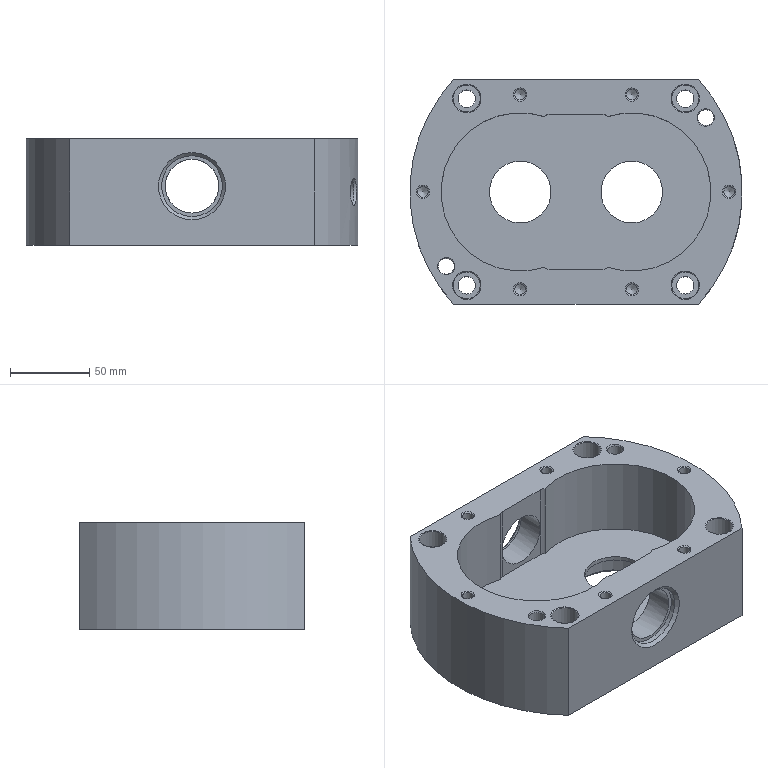NC program | NX | posted with a generic post | part box 210 x 142 x 67.4 mm
Lines 526 to 1432 of 22889:
(FLOOR_WALL_1_1 , TOOL : D25R0.5)
N1032 T05 M6
N1034 G54
N1036 G17 G0 G90 X-2.853 Y1.35 B0. C0. S2000 M3
N1038 G43 Z30. H5
N1040 Z1.5
N1042 G94 G1 X-8.606 Z1.349 F1000.
N1044 X-9.554 Y1.117 Z1.324
N1046 X-12.104 Y0.616 Z1.256
N1048 X-14.678 Y0.256 Z1.188
N1050 X-17.268 Y0.036 Z1.12
N1052 X-18.244 Y0. Z1.094
N1054 X-17.268 Y-0.036 Z1.068
N1056 X-14.678 Y-0.256 Z1.
N1058 X-12.104 Y-0.616 Z0.932
N1060 X-9.554 Y-1.117 Z0.864
N1062 X-8.606 Y-1.35 Z0.839
N1064 X8.606 Z0.388
N1066 X9.554 Y-1.117 Z0.362
N1068 X12.104 Y-0.616 Z0.294
N1070 X14.678 Y-0.256 Z0.226
N1072 X17.268 Y-0.036 Z0.158
N1074 X18.244 Y0. Z0.133
N1076 X17.268 Y0.036 Z0.107
N1078 X14.678 Y0.256 Z0.039
N1080 X12.104 Y0.616 Z-0.029
N1082 X9.554 Y1.117 Z-0.097
N1084 X8.606 Y1.35 Z-0.123
N1086 X0. Z-0.348
N1088 X-8.606 F2200.
N1090 G2 X-18.244 Y0. R47.65
N1092 X-8.606 Y-1.35 R47.65
N1094 G1 X8.606
N1096 G2 X18.244 Y0. R47.65
N1098 X8.606 Y1.35 R47.65
N1100 G1 X0.
N1102 Y18.85
N1104 X-10.975
N1106 G2 X-21.111 Y17.488 R30.15
N1108 G1 X-21.756 Y0.
N1110 G2 X-34.533 Y2.238 R47.65
N1112 G3 X-34.533 Y-2.238 R-2.35
N1114 G2 X-21.756 Y0. R47.65
N1116 G1 X-21.111 Y17.488
N1118 G2 X-29.196 Y18.904 R30.15
N1120 G3 X-29.196 Y-18.904 R-19.85
N1122 G2 X-10.975 Y-18.85 R30.15
N1124 G1 X10.975
N1126 G2 X21.111 Y-17.488 R30.15
N1128 G1 X21.756 Y0.
N1130 G2 X34.533 Y-2.238 R47.65
N1132 G3 X34.533 Y2.238 R-2.35
N1134 G2 X21.756 Y0. R47.65
N1136 G1 X21.111 Y-17.488
N1138 G2 X29.196 Y-18.904 R30.15
N1140 G3 X29.196 Y18.904 R-19.85
N1142 G2 X10.975 Y18.85 R30.15
N1144 G1 X0.
N1146 Y36.35
N1148 X-14.25
N1150 G2 X-23.858 Y35.57 R12.65
N1152 G3 X-23.858 Y-35.57 R-37.35
N1154 G2 X-14.25 Y-36.35 R12.65
N1156 G1 X14.25
N1158 G2 X23.858 Y-35.57 R12.65
N1160 G3 X23.858 Y35.57 R-37.35
N1162 G2 X14.25 Y36.35 R12.65
N1164 G1 X0.
N1166 Z1.152
N1168 G0 X-2.853 Y1.35
N1170 G1 X-8.606 Z1.001 F1000.
N1172 X-9.554 Y1.117 Z0.976
N1174 X-12.104 Y0.616 Z0.908
N1176 X-14.678 Y0.256 Z0.84
N1178 X-17.268 Y0.036 Z0.772
N1180 X-18.244 Y0. Z0.746
N1182 X-17.268 Y-0.036 Z0.721
N1184 X-14.678 Y-0.256 Z0.653
N1186 X-12.104 Y-0.616 Z0.584
N1188 X-9.554 Y-1.117 Z0.516
N1190 X-8.606 Y-1.35 Z0.491
N1192 X8.606 Z0.04
N1194 X9.554 Y-1.117 Z0.015
N1196 X12.104 Y-0.616 Z-0.053
N1198 X14.678 Y-0.256 Z-0.122
N1200 X17.268 Y-0.036 Z-0.19
N1202 X18.244 Y0. Z-0.215
N1204 X17.268 Y0.036 Z-0.241
N1206 X14.678 Y0.256 Z-0.309
N1208 X12.104 Y0.616 Z-0.377
N1210 X9.554 Y1.117 Z-0.445
N1212 X8.606 Y1.35 Z-0.47
N1214 X0. Z-0.696
N1216 X-8.606 F2200.
N1218 G2 X-18.244 Y0. R47.65
N1220 X-8.606 Y-1.35 R47.65
N1222 G1 X8.606
N1224 G2 X18.244 Y0. R47.65
N1226 X8.606 Y1.35 R47.65
N1228 G1 X0.
N1230 Y18.85
N1232 X-10.975
N1234 G2 X-21.111 Y17.488 R30.15
N1236 G1 X-21.756 Y0.
N1238 G2 X-34.533 Y2.238 R47.65
N1240 G3 X-34.533 Y-2.238 R-2.35
N1242 G2 X-21.756 Y0. R47.65
N1244 G1 X-21.111 Y17.488
N1246 G2 X-29.196 Y18.904 R30.15
N1248 G3 X-29.196 Y-18.904 R-19.85
N1250 G2 X-10.975 Y-18.85 R30.15
N1252 G1 X10.975
N1254 G2 X21.111 Y-17.488 R30.15
N1256 G1 X21.756 Y0.
N1258 G2 X34.533 Y-2.238 R47.65
N1260 G3 X34.533 Y2.238 R-2.35
N1262 G2 X21.756 Y0. R47.65
N1264 G1 X21.111 Y-17.488
N1266 G2 X29.196 Y-18.904 R30.15
N1268 G3 X29.196 Y18.904 R-19.85
N1270 G2 X10.975 Y18.85 R30.15
N1272 G1 X0.
N1274 Y36.35
N1276 X-14.25
N1278 G2 X-23.858 Y35.57 R12.65
N1280 G3 X-23.858 Y-35.57 R-37.35
N1282 G2 X-14.25 Y-36.35 R12.65
N1284 G1 X14.25
N1286 G2 X23.858 Y-35.57 R12.65
N1288 G3 X23.858 Y35.57 R-37.35
N1290 G2 X14.25 Y36.35 R12.65
N1292 G1 X0.
N1294 Z0.804
N1296 G0 X-2.853 Y1.35
N1298 G1 X-8.606 Z0.654 F1000.
N1300 X-9.554 Y1.117 Z0.628
N1302 X-12.104 Y0.616 Z0.56
N1304 X-14.678 Y0.256 Z0.492
N1306 X-17.268 Y0.036 Z0.424
N1308 X-18.244 Y0. Z0.398
N1310 X-17.268 Y-0.036 Z0.373
N1312 X-14.678 Y-0.256 Z0.305
N1314 X-12.104 Y-0.616 Z0.237
N1316 X-9.554 Y-1.117 Z0.168
N1318 X-8.606 Y-1.35 Z0.143
N1320 X8.606 Z-0.308
N1322 X9.554 Y-1.117 Z-0.333
N1324 X12.104 Y-0.616 Z-0.401
N1326 X14.678 Y-0.256 Z-0.469
N1328 X17.268 Y-0.036 Z-0.538
N1330 X18.244 Y0. Z-0.563
N1332 X17.268 Y0.036 Z-0.589
N1334 X14.678 Y0.256 Z-0.657
N1336 X12.104 Y0.616 Z-0.725
N1338 X9.554 Y1.117 Z-0.793
N1340 X8.606 Y1.35 Z-0.818
N1342 X0. Z-1.044
N1344 X-8.606 F2200.
N1346 G2 X-18.244 Y0. R47.65
N1348 X-8.606 Y-1.35 R47.65
N1350 G1 X8.606
N1352 G2 X18.244 Y0. R47.65
N1354 X8.606 Y1.35 R47.65
N1356 G1 X0.
N1358 Y18.85
N1360 X-10.975
N1362 G2 X-21.111 Y17.488 R30.15
N1364 G1 X-21.756 Y0.
N1366 G2 X-34.533 Y2.238 R47.65
N1368 G3 X-34.533 Y-2.238 R-2.35
N1370 G2 X-21.756 Y0. R47.65
N1372 G1 X-21.111 Y17.488
N1374 G2 X-29.196 Y18.904 R30.15
N1376 G3 X-29.196 Y-18.904 R-19.85
N1378 G2 X-10.975 Y-18.85 R30.15
N1380 G1 X10.975
N1382 G2 X21.111 Y-17.488 R30.15
N1384 G1 X21.756 Y0.
N1386 G2 X34.533 Y-2.238 R47.65
N1388 G3 X34.533 Y2.238 R-2.35
N1390 G2 X21.756 Y0. R47.65
N1392 G1 X21.111 Y-17.488
N1394 G2 X29.196 Y-18.904 R30.15
N1396 G3 X29.196 Y18.904 R-19.85
N1398 G2 X10.975 Y18.85 R30.15
N1400 G1 X0.
N1402 Y36.35
N1404 X-14.25
N1406 G2 X-23.858 Y35.57 R12.65
N1408 G3 X-23.858 Y-35.57 R-37.35
N1410 G2 X-14.25 Y-36.35 R12.65
N1412 G1 X14.25
N1414 G2 X23.858 Y-35.57 R12.65
N1416 G3 X23.858 Y35.57 R-37.35
N1418 G2 X14.25 Y36.35 R12.65
N1420 G1 X0.
N1422 Z0.456
N1424 G0 X-2.853 Y1.35
N1426 G1 X-8.606 Z0.306 F1000.
N1428 X-9.554 Y1.117 Z0.28
N1430 X-12.104 Y0.616 Z0.212
N1432 X-14.678 Y0.256 Z0.144
N1434 X-17.268 Y0.036 Z0.076
N1436 X-18.244 Y0. Z0.05
N1438 X-17.268 Y-0.036 Z0.025
N1440 X-14.678 Y-0.256 Z-0.043
N1442 X-12.104 Y-0.616 Z-0.111
N1444 X-9.554 Y-1.117 Z-0.179
N1446 X-8.606 Y-1.35 Z-0.205
N1448 X8.606 Z-0.656
N1450 X9.554 Y-1.117 Z-0.681
N1452 X12.104 Y-0.616 Z-0.749
N1454 X14.678 Y-0.256 Z-0.817
N1456 X17.268 Y-0.036 Z-0.885
N1458 X18.244 Y0. Z-0.911
N1460 X17.268 Y0.036 Z-0.937
N1462 X14.678 Y0.256 Z-1.005
N1464 X12.104 Y0.616 Z-1.073
N1466 X9.554 Y1.117 Z-1.141
N1468 X8.606 Y1.35 Z-1.166
N1470 X0. Z-1.392
N1472 X-8.606 F2200.
N1474 G2 X-18.244 Y0. R47.65
N1476 X-8.606 Y-1.35 R47.65
N1478 G1 X8.606
N1480 G2 X18.244 Y0. R47.65
N1482 X8.606 Y1.35 R47.65
N1484 G1 X0.
N1486 Y18.85
N1488 X-10.975
N1490 G2 X-21.111 Y17.488 R30.15
N1492 G1 X-21.756 Y0.
N1494 G2 X-34.533 Y2.238 R47.65
N1496 G3 X-34.533 Y-2.238 R-2.35
N1498 G2 X-21.756 Y0. R47.65
N1500 G1 X-21.111 Y17.488
N1502 G2 X-29.196 Y18.904 R30.15
N1504 G3 X-29.196 Y-18.904 R-19.85
N1506 G2 X-10.975 Y-18.85 R30.15
N1508 G1 X10.975
N1510 G2 X21.111 Y-17.488 R30.15
N1512 G1 X21.756 Y0.
N1514 G2 X34.533 Y-2.238 R47.65
N1516 G3 X34.533 Y2.238 R-2.35
N1518 G2 X21.756 Y0. R47.65
N1520 G1 X21.111 Y-17.488
N1522 G2 X29.196 Y-18.904 R30.15
N1524 G3 X29.196 Y18.904 R-19.85
N1526 G2 X10.975 Y18.85 R30.15
N1528 G1 X0.
N1530 Y36.35
N1532 X-14.25
N1534 G2 X-23.858 Y35.57 R12.65
N1536 G3 X-23.858 Y-35.57 R-37.35
N1538 G2 X-14.25 Y-36.35 R12.65
N1540 G1 X14.25
N1542 G2 X23.858 Y-35.57 R12.65
N1544 G3 X23.858 Y35.57 R-37.35
N1546 G2 X14.25 Y36.35 R12.65
N1548 G1 X0.
N1550 Z0.108
N1552 G0 X-2.853 Y1.35
N1554 G1 X-8.606 Z-0.042 F1000.
N1556 X-9.554 Y1.117 Z-0.068
N1558 X-12.104 Y0.616 Z-0.136
N1560 X-14.678 Y0.256 Z-0.204
N1562 X-17.268 Y0.036 Z-0.272
N1564 X-18.244 Y0. Z-0.298
N1566 X-17.268 Y-0.036 Z-0.323
N1568 X-14.678 Y-0.256 Z-0.391
N1570 X-12.104 Y-0.616 Z-0.459
N1572 X-9.554 Y-1.117 Z-0.527
N1574 X-8.606 Y-1.35 Z-0.553
N1576 X8.606 Z-1.004
N1578 X9.554 Y-1.117 Z-1.029
N1580 X12.104 Y-0.616 Z-1.097
N1582 X14.678 Y-0.256 Z-1.165
N1584 X17.268 Y-0.036 Z-1.233
N1586 X18.244 Y0. Z-1.259
N1588 X17.268 Y0.036 Z-1.284
N1590 X14.678 Y0.256 Z-1.353
N1592 X12.104 Y0.616 Z-1.421
N1594 X9.554 Y1.117 Z-1.489
N1596 X8.606 Y1.35 Z-1.514
N1598 X0. Z-1.74
N1600 X-8.606 F2200.
N1602 G2 X-18.244 Y0. R47.65
N1604 X-8.606 Y-1.35 R47.65
N1606 G1 X8.606
N1608 G2 X18.244 Y0. R47.65
N1610 X8.606 Y1.35 R47.65
N1612 G1 X0.
N1614 Y18.85
N1616 X-10.975
N1618 G2 X-21.111 Y17.488 R30.15
N1620 G1 X-21.756 Y0.
N1622 G2 X-34.533 Y2.238 R47.65
N1624 G3 X-34.533 Y-2.238 R-2.35
N1626 G2 X-21.756 Y0. R47.65
N1628 G1 X-21.111 Y17.488
N1630 G2 X-29.196 Y18.904 R30.15
N1632 G3 X-29.196 Y-18.904 R-19.85
N1634 G2 X-10.975 Y-18.85 R30.15
N1636 G1 X10.975
N1638 G2 X21.111 Y-17.488 R30.15
N1640 G1 X21.756 Y0.
N1642 G2 X34.533 Y-2.238 R47.65
N1644 G3 X34.533 Y2.238 R-2.35
N1646 G2 X21.756 Y0. R47.65
N1648 G1 X21.111 Y-17.488
N1650 G2 X29.196 Y-18.904 R30.15
N1652 G3 X29.196 Y18.904 R-19.85
N1654 G2 X10.975 Y18.85 R30.15
N1656 G1 X0.
N1658 Y36.35
N1660 X-14.25
N1662 G2 X-23.858 Y35.57 R12.65
N1664 G3 X-23.858 Y-35.57 R-37.35
N1666 G2 X-14.25 Y-36.35 R12.65
N1668 G1 X14.25
N1670 G2 X23.858 Y-35.57 R12.65
N1672 G3 X23.858 Y35.57 R-37.35
N1674 G2 X14.25 Y36.35 R12.65
N1676 G1 X0.
N1678 Z-0.24
N1680 G0 X-2.853 Y1.35
N1682 G1 X-8.606 Z-0.39 F1000.
N1684 X-9.554 Y1.117 Z-0.416
N1686 X-12.104 Y0.616 Z-0.484
N1688 X-14.678 Y0.256 Z-0.552
N1690 X-17.268 Y0.036 Z-0.62
N1692 X-18.244 Y0. Z-0.646
N1694 X-17.268 Y-0.036 Z-0.671
N1696 X-14.678 Y-0.256 Z-0.739
N1698 X-12.104 Y-0.616 Z-0.807
N1700 X-9.554 Y-1.117 Z-0.875
N1702 X-8.606 Y-1.35 Z-0.901
N1704 X8.606 Z-1.352
N1706 X9.554 Y-1.117 Z-1.377
N1708 X12.104 Y-0.616 Z-1.445
N1710 X14.678 Y-0.256 Z-1.513
N1712 X17.268 Y-0.036 Z-1.581
N1714 X18.244 Y0. Z-1.607
N1716 X17.268 Y0.036 Z-1.632
N1718 X14.678 Y0.256 Z-1.7
N1720 X12.104 Y0.616 Z-1.769
N1722 X9.554 Y1.117 Z-1.837
N1724 X8.606 Y1.35 Z-1.862
N1726 X0. Z-2.088
N1728 X-8.606 F2200.
N1730 G2 X-18.244 Y0. R47.65
N1732 X-8.606 Y-1.35 R47.65
N1734 G1 X8.606
N1736 G2 X18.244 Y0. R47.65
N1738 X8.606 Y1.35 R47.65
N1740 G1 X0.
N1742 Y18.85
N1744 X-10.975
N1746 G2 X-21.111 Y17.488 R30.15
N1748 G1 X-21.756 Y0.
N1750 G2 X-34.533 Y2.238 R47.65
N1752 G3 X-34.533 Y-2.238 R-2.35
N1754 G2 X-21.756 Y0. R47.65
N1756 G1 X-21.111 Y17.488
N1758 G2 X-29.196 Y18.904 R30.15
N1760 G3 X-29.196 Y-18.904 R-19.85
N1762 G2 X-10.975 Y-18.85 R30.15
N1764 G1 X10.975
N1766 G2 X21.111 Y-17.488 R30.15
N1768 G1 X21.756 Y0.
N1770 G2 X34.533 Y-2.238 R47.65
N1772 G3 X34.533 Y2.238 R-2.35
N1774 G2 X21.756 Y0. R47.65
N1776 G1 X21.111 Y-17.488
N1778 G2 X29.196 Y-18.904 R30.15
N1780 G3 X29.196 Y18.904 R-19.85
N1782 G2 X10.975 Y18.85 R30.15
N1784 G1 X0.
N1786 Y36.35
N1788 X-14.25
N1790 G2 X-23.858 Y35.57 R12.65
N1792 G3 X-23.858 Y-35.57 R-37.35
N1794 G2 X-14.25 Y-36.35 R12.65
N1796 G1 X14.25
N1798 G2 X23.858 Y-35.57 R12.65
N1800 G3 X23.858 Y35.57 R-37.35
N1802 G2 X14.25 Y36.35 R12.65
N1804 G1 X0.
N1806 Z-0.588
N1808 G0 X-2.853 Y1.35
N1810 G1 X-8.606 Z-0.738 F1000.
N1812 X-9.554 Y1.117 Z-0.764
N1814 X-12.104 Y0.616 Z-0.832
N1816 X-14.678 Y0.256 Z-0.9
N1818 X-17.268 Y0.036 Z-0.968
N1820 X-18.244 Y0. Z-0.993
N1822 X-17.268 Y-0.036 Z-1.019
N1824 X-14.678 Y-0.256 Z-1.087
N1826 X-12.104 Y-0.616 Z-1.155
N1828 X-9.554 Y-1.117 Z-1.223
N1830 X-8.606 Y-1.35 Z-1.249
N1832 X8.606 Z-1.699
N1834 X9.554 Y-1.117 Z-1.725
N1836 X12.104 Y-0.616 Z-1.793
N1838 X14.678 Y-0.256 Z-1.861
N1840 X17.268 Y-0.036 Z-1.929
N1842 X18.244 Y0. Z-1.955
N1844 X17.268 Y0.036 Z-1.98
N1846 X14.678 Y0.256 Z-2.048
N1848 X12.104 Y0.616 Z-2.116
N1850 X9.554 Y1.117 Z-2.185
N1852 X8.606 Y1.35 Z-2.21
N1854 X0. Z-2.435
N1856 X-8.606 F2200.
N1858 G2 X-18.244 Y0. R47.65
N1860 X-8.606 Y-1.35 R47.65
N1862 G1 X8.606
N1864 G2 X18.244 Y0. R47.65
N1866 X8.606 Y1.35 R47.65
N1868 G1 X0.
N1870 Y18.85
N1872 X-10.975
N1874 G2 X-21.111 Y17.488 R30.15
N1876 G1 X-21.756 Y0.
N1878 G2 X-34.533 Y2.238 R47.65
N1880 G3 X-34.533 Y-2.238 R-2.35
N1882 G2 X-21.756 Y0. R47.65
N1884 G1 X-21.111 Y17.488
N1886 G2 X-29.196 Y18.904 R30.15
N1888 G3 X-29.196 Y-18.904 R-19.85
N1890 G2 X-10.975 Y-18.85 R30.15
N1892 G1 X10.975
N1894 G2 X21.111 Y-17.488 R30.15
N1896 G1 X21.756 Y0.
N1898 G2 X34.533 Y-2.238 R47.65
N1900 G3 X34.533 Y2.238 R-2.35
N1902 G2 X21.756 Y0. R47.65
N1904 G1 X21.111 Y-17.488
N1906 G2 X29.196 Y-18.904 R30.15
N1908 G3 X29.196 Y18.904 R-19.85
N1910 G2 X10.975 Y18.85 R30.15
N1912 G1 X0.
N1914 Y36.35
N1916 X-14.25
N1918 G2 X-23.858 Y35.57 R12.65
N1920 G3 X-23.858 Y-35.57 R-37.35
N1922 G2 X-14.25 Y-36.35 R12.65
N1924 G1 X14.25
N1926 G2 X23.858 Y-35.57 R12.65
N1928 G3 X23.858 Y35.57 R-37.35
N1930 G2 X14.25 Y36.35 R12.65
N1932 G1 X0.
N1934 Z-0.935
N1936 G0 X-2.853 Y1.35
N1938 G1 X-8.606 Z-1.086 F1000.
N1940 X-9.554 Y1.117 Z-1.112
N1942 X-12.104 Y0.616 Z-1.18
N1944 X-14.678 Y0.256 Z-1.248
N1946 X-17.268 Y0.036 Z-1.316
N1948 X-18.244 Y0. Z-1.341
N1950 X-17.268 Y-0.036 Z-1.367
N1952 X-14.678 Y-0.256 Z-1.435
N1954 X-12.104 Y-0.616 Z-1.503
N1956 X-9.554 Y-1.117 Z-1.571
N1958 X-8.606 Y-1.35 Z-1.597
N1960 X8.606 Z-2.047
N1962 X9.554 Y-1.117 Z-2.073
N1964 X12.104 Y-0.616 Z-2.141
N1966 X14.678 Y-0.256 Z-2.209
N1968 X17.268 Y-0.036 Z-2.277
N1970 X18.244 Y0. Z-2.303
N1972 X17.268 Y0.036 Z-2.328
N1974 X14.678 Y0.256 Z-2.396
N1976 X12.104 Y0.616 Z-2.464
N1978 X9.554 Y1.117 Z-2.532
N1980 X8.606 Y1.35 Z-2.558
N1982 X0. Z-2.783
N1984 X-8.606 F2200.
N1986 G2 X-18.244 Y0. R47.65
N1988 X-8.606 Y-1.35 R47.65
N1990 G1 X8.606
N1992 G2 X18.244 Y0. R47.65
N1994 X8.606 Y1.35 R47.65
N1996 G1 X0.
N1998 Y18.85
N2000 X-10.975
N2002 G2 X-21.111 Y17.488 R30.15
N2004 G1 X-21.756 Y0.
N2006 G2 X-34.533 Y2.238 R47.65
N2008 G3 X-34.533 Y-2.238 R-2.35
N2010 G2 X-21.756 Y0. R47.65
N2012 G1 X-21.111 Y17.488
N2014 G2 X-29.196 Y18.904 R30.15
N2016 G3 X-29.196 Y-18.904 R-19.85
N2018 G2 X-10.975 Y-18.85 R30.15
N2020 G1 X10.975
N2022 G2 X21.111 Y-17.488 R30.15
N2024 G1 X21.756 Y0.
N2026 G2 X34.533 Y-2.238 R47.65
N2028 G3 X34.533 Y2.238 R-2.35
N2030 G2 X21.756 Y0. R47.65
N2032 G1 X21.111 Y-17.488
N2034 G2 X29.196 Y-18.904 R30.15
N2036 G3 X29.196 Y18.904 R-19.85
N2038 G2 X10.975 Y18.85 R30.15
N2040 G1 X0.
N2042 Y36.35
N2044 X-14.25
N2046 G2 X-23.858 Y35.57 R12.65
N2048 G3 X-23.858 Y-35.57 R-37.35
N2050 G2 X-14.25 Y-36.35 R12.65
N2052 G1 X14.25
N2054 G2 X23.858 Y-35.57 R12.65
N2056 G3 X23.858 Y35.57 R-37.35
N2058 G2 X14.25 Y36.35 R12.65
N2060 G1 X0.
N2062 Z-1.283
N2064 G0 X-2.853 Y1.35
N2066 G1 X-8.606 Z-1.434 F1000.
N2068 X-9.554 Y1.117 Z-1.46
N2070 X-12.104 Y0.616 Z-1.528
N2072 X-14.678 Y0.256 Z-1.596
N2074 X-17.268 Y0.036 Z-1.664
N2076 X-18.244 Y0. Z-1.689
N2078 X-17.268 Y-0.036 Z-1.715
N2080 X-14.678 Y-0.256 Z-1.783
N2082 X-12.104 Y-0.616 Z-1.851
N2084 X-9.554 Y-1.117 Z-1.919
N2086 X-8.606 Y-1.35 Z-1.945
N2088 X8.606 Z-2.395
N2090 X9.554 Y-1.117 Z-2.421
N2092 X12.104 Y-0.616 Z-2.489
N2094 X14.678 Y-0.256 Z-2.557
N2096 X17.268 Y-0.036 Z-2.625
N2098 X18.244 Y0. Z-2.651
N2100 X17.268 Y0.036 Z-2.676
N2102 X14.678 Y0.256 Z-2.744
N2104 X12.104 Y0.616 Z-2.812
N2106 X9.554 Y1.117 Z-2.88
N2108 X8.606 Y1.35 Z-2.906
N2110 X0. Z-3.131
N2112 X-8.606 F2200.
N2114 G2 X-18.244 Y0. R47.65
N2116 X-8.606 Y-1.35 R47.65
N2118 G1 X8.606
N2120 G2 X18.244 Y0. R47.65
N2122 X8.606 Y1.35 R47.65
N2124 G1 X0.
N2126 Y18.85
N2128 X-10.975
N2130 G2 X-21.111 Y17.488 R30.15
N2132 G1 X-21.756 Y0.
N2134 G2 X-34.533 Y2.238 R47.65
N2136 G3 X-34.533 Y-2.238 R-2.35
N2138 G2 X-21.756 Y0. R47.65
N2140 G1 X-21.111 Y17.488
N2142 G2 X-29.196 Y18.904 R30.15
N2144 G3 X-29.196 Y-18.904 R-19.85
N2146 G2 X-10.975 Y-18.85 R30.15
N2148 G1 X10.975
N2150 G2 X21.111 Y-17.488 R30.15
N2152 G1 X21.756 Y0.
N2154 G2 X34.533 Y-2.238 R47.65
N2156 G3 X34.533 Y2.238 R-2.35
N2158 G2 X21.756 Y0. R47.65
N2160 G1 X21.111 Y-17.488
N2162 G2 X29.196 Y-18.904 R30.15
N2164 G3 X29.196 Y18.904 R-19.85
N2166 G2 X10.975 Y18.85 R30.15
N2168 G1 X0.
N2170 Y36.35
N2172 X-14.25
N2174 G2 X-23.858 Y35.57 R12.65
N2176 G3 X-23.858 Y-35.57 R-37.35
N2178 G2 X-14.25 Y-36.35 R12.65
N2180 G1 X14.25
N2182 G2 X23.858 Y-35.57 R12.65
N2184 G3 X23.858 Y35.57 R-37.35
N2186 G2 X14.25 Y36.35 R12.65
N2188 G1 X0.
N2190 Z-1.631
N2192 G0 X-2.853 Y1.35
N2194 G1 X-8.606 Z-1.782 F1000.
N2196 X-9.554 Y1.117 Z-1.807
N2198 X-12.104 Y0.616 Z-1.876
N2200 X-14.678 Y0.256 Z-1.944
N2202 X-17.268 Y0.036 Z-2.012
N2204 X-18.244 Y0. Z-2.037
N2206 X-17.268 Y-0.036 Z-2.063
N2208 X-14.678 Y-0.256 Z-2.131
N2210 X-12.104 Y-0.616 Z-2.199
N2212 X-9.554 Y-1.117 Z-2.267
N2214 X-8.606 Y-1.35 Z-2.293
N2216 X8.606 Z-2.743
N2218 X9.554 Y-1.117 Z-2.769
N2220 X12.104 Y-0.616 Z-2.837
N2222 X14.678 Y-0.256 Z-2.905
N2224 X17.268 Y-0.036 Z-2.973
N2226 X18.244 Y0. Z-2.999
N2228 X17.268 Y0.036 Z-3.024
N2230 X14.678 Y0.256 Z-3.092
N2232 X12.104 Y0.616 Z-3.16
N2234 X9.554 Y1.117 Z-3.228
N2236 X8.606 Y1.35 Z-3.254
N2238 X0. Z-3.479
N2240 X-8.606 F2200.
N2242 G2 X-18.244 Y0. R47.65
N2244 X-8.606 Y-1.35 R47.65
N2246 G1 X8.606
N2248 G2 X18.244 Y0. R47.65
N2250 X8.606 Y1.35 R47.65
N2252 G1 X0.
N2254 Y18.85
N2256 X-10.975
N2258 G2 X-21.111 Y17.488 R30.15
N2260 G1 X-21.756 Y0.
N2262 G2 X-34.533 Y2.238 R47.65
N2264 G3 X-34.533 Y-2.238 R-2.35
N2266 G2 X-21.756 Y0. R47.65
N2268 G1 X-21.111 Y17.488
N2270 G2 X-29.196 Y18.904 R30.15
N2272 G3 X-29.196 Y-18.904 R-19.85
N2274 G2 X-10.975 Y-18.85 R30.15
N2276 G1 X10.975
N2278 G2 X21.111 Y-17.488 R30.15
N2280 G1 X21.756 Y0.
N2282 G2 X34.533 Y-2.238 R47.65
N2284 G3 X34.533 Y2.238 R-2.35
N2286 G2 X21.756 Y0. R47.65
N2288 G1 X21.111 Y-17.488
N2290 G2 X29.196 Y-18.904 R30.15
N2292 G3 X29.196 Y18.904 R-19.85
N2294 G2 X10.975 Y18.85 R30.15
N2296 G1 X0.
N2298 Y36.35
N2300 X-14.25
N2302 G2 X-23.858 Y35.57 R12.65
N2304 G3 X-23.858 Y-35.57 R-37.35
N2306 G2 X-14.25 Y-36.35 R12.65
N2308 G1 X14.25
N2310 G2 X23.858 Y-35.57 R12.65
N2312 G3 X23.858 Y35.57 R-37.35
N2314 G2 X14.25 Y36.35 R12.65
N2316 G1 X0.
N2318 Z-1.979
N2320 G0 X-2.853 Y1.35
N2322 G1 X-8.606 Z-2.13 F1000.
N2324 X-9.554 Y1.117 Z-2.155
N2326 X-12.104 Y0.616 Z-2.223
N2328 X-14.678 Y0.256 Z-2.291
N2330 X-17.268 Y0.036 Z-2.36
N2332 X-18.244 Y0. Z-2.385
N2334 X-17.268 Y-0.036 Z-2.411
N2336 X-14.678 Y-0.256 Z-2.479
N2338 X-12.104 Y-0.616 Z-2.547
N2340 X-9.554 Y-1.117 Z-2.615
N2342 X-8.606 Y-1.35 Z-2.64
N2344 X8.606 Z-3.091
N2346 X9.554 Y-1.117 Z-3.117
N2348 X12.104 Y-0.616 Z-3.185
N2350 X14.678 Y-0.256 Z-3.253
N2352 X17.268 Y-0.036 Z-3.321
N2354 X18.244 Y0. Z-3.346
N2356 X17.268 Y0.036 Z-3.372
N2358 X14.678 Y0.256 Z-3.44
N2360 X12.104 Y0.616 Z-3.508
N2362 X9.554 Y1.117 Z-3.576
N2364 X8.606 Y1.35 Z-3.602
N2366 X0. Z-3.827
N2368 X-8.606 F2200.
N2370 G2 X-18.244 Y0. R47.65
N2372 X-8.606 Y-1.35 R47.65
N2374 G1 X8.606
N2376 G2 X18.244 Y0. R47.65
N2378 X8.606 Y1.35 R47.65
N2380 G1 X0.
N2382 Y18.85
N2384 X-10.975
N2386 G2 X-21.111 Y17.488 R30.15
N2388 G1 X-21.756 Y0.
N2390 G2 X-34.533 Y2.238 R47.65
N2392 G3 X-34.533 Y-2.238 R-2.35
N2394 G2 X-21.756 Y0. R47.65
N2396 G1 X-21.111 Y17.488
N2398 G2 X-29.196 Y18.904 R30.15
N2400 G3 X-29.196 Y-18.904 R-19.85
N2402 G2 X-10.975 Y-18.85 R30.15
N2404 G1 X10.975
N2406 G2 X21.111 Y-17.488 R30.15
N2408 G1 X21.756 Y0.
N2410 G2 X34.533 Y-2.238 R47.65
N2412 G3 X34.533 Y2.238 R-2.35
N2414 G2 X21.756 Y0. R47.65
N2416 G1 X21.111 Y-17.488
N2418 G2 X29.196 Y-18.904 R30.15
N2420 G3 X29.196 Y18.904 R-19.85
N2422 G2 X10.975 Y18.85 R30.15
N2424 G1 X0.
N2426 Y36.35
N2428 X-14.25
N2430 G2 X-23.858 Y35.57 R12.65
N2432 G3 X-23.858 Y-35.57 R-37.35
N2434 G2 X-14.25 Y-36.35 R12.65
N2436 G1 X14.25
N2438 G2 X23.858 Y-35.57 R12.65
N2440 G3 X23.858 Y35.57 R-37.35
N2442 G2 X14.25 Y36.35 R12.65
N2444 G1 X0.
N2446 Z-2.327
N2448 G0 X-2.853 Y1.35
N2450 G1 X-8.606 Z-2.478 F1000.
N2452 X-9.554 Y1.117 Z-2.503
N2454 X-12.104 Y0.616 Z-2.571
N2456 X-14.678 Y0.256 Z-2.639
N2458 X-17.268 Y0.036 Z-2.707
N2460 X-18.244 Y0. Z-2.733
N2462 X-17.268 Y-0.036 Z-2.759
N2464 X-14.678 Y-0.256 Z-2.827
N2466 X-12.104 Y-0.616 Z-2.895
N2468 X-9.554 Y-1.117 Z-2.963
N2470 X-8.606 Y-1.35 Z-2.988
N2472 X8.606 Z-3.439
N2474 X9.554 Y-1.117 Z-3.465
N2476 X12.104 Y-0.616 Z-3.533
N2478 X14.678 Y-0.256 Z-3.601
N2480 X17.268 Y-0.036 Z-3.669
N2482 X18.244 Y0. Z-3.694
N2484 X17.268 Y0.036 Z-3.72
N2486 X14.678 Y0.256 Z-3.788
N2488 X12.104 Y0.616 Z-3.856
N2490 X9.554 Y1.117 Z-3.924
N2492 X8.606 Y1.35 Z-3.95
N2494 X0. Z-4.175
N2496 X-8.606 F2200.
N2498 G2 X-18.244 Y0. R47.65
N2500 X-8.606 Y-1.35 R47.65
N2502 G1 X8.606
N2504 G2 X18.244 Y0. R47.65
N2506 X8.606 Y1.35 R47.65
N2508 G1 X0.
N2510 Y18.85
N2512 X-10.975
N2514 G2 X-21.111 Y17.488 R30.15
N2516 G1 X-21.756 Y0.
N2518 G2 X-34.533 Y2.238 R47.65
N2520 G3 X-34.533 Y-2.238 R-2.35
N2522 G2 X-21.756 Y0. R47.65
N2524 G1 X-21.111 Y17.488
N2526 G2 X-29.196 Y18.904 R30.15
N2528 G3 X-29.196 Y-18.904 R-19.85
N2530 G2 X-10.975 Y-18.85 R30.15
N2532 G1 X10.975
N2534 G2 X21.111 Y-17.488 R30.15
N2536 G1 X21.756 Y0.
N2538 G2 X34.533 Y-2.238 R47.65
N2540 G3 X34.533 Y2.238 R-2.35
N2542 G2 X21.756 Y0. R47.65
N2544 G1 X21.111 Y-17.488
N2546 G2 X29.196 Y-18.904 R30.15
N2548 G3 X29.196 Y18.904 R-19.85
N2550 G2 X10.975 Y18.85 R30.15
N2552 G1 X0.
N2554 Y36.35
N2556 X-14.25
N2558 G2 X-23.858 Y35.57 R12.65
N2560 G3 X-23.858 Y-35.57 R-37.35
N2562 G2 X-14.25 Y-36.35 R12.65
N2564 G1 X14.25
N2566 G2 X23.858 Y-35.57 R12.65
N2568 G3 X23.858 Y35.57 R-37.35
N2570 G2 X14.25 Y36.35 R12.65
N2572 G1 X0.
N2574 Z-2.675
N2576 G0 X-2.853 Y1.35
N2578 G1 X-8.606 Z-2.826 F1000.
N2580 X-9.554 Y1.117 Z-2.851
N2582 X-12.104 Y0.616 Z-2.919
N2584 X-14.678 Y0.256 Z-2.987
N2586 X-17.268 Y0.036 Z-3.055
N2588 X-18.244 Y0. Z-3.081
N2590 X-17.268 Y-0.036 Z-3.107
N2592 X-14.678 Y-0.256 Z-3.175
N2594 X-12.104 Y-0.616 Z-3.243
N2596 X-9.554 Y-1.117 Z-3.311
N2598 X-8.606 Y-1.35 Z-3.336
N2600 X8.606 Z-3.787
N2602 X9.554 Y-1.117 Z-3.813
N2604 X12.104 Y-0.616 Z-3.881
N2606 X14.678 Y-0.256 Z-3.949
N2608 X17.268 Y-0.036 Z-4.017
N2610 X18.244 Y0. Z-4.042
N2612 X17.268 Y0.036 Z-4.068
N2614 X14.678 Y0.256 Z-4.136
N2616 X12.104 Y0.616 Z-4.204
N2618 X9.554 Y1.117 Z-4.272
N2620 X8.606 Y1.35 Z-4.298
N2622 X0. Z-4.523
N2624 X-8.606 F2200.
N2626 G2 X-18.244 Y0. R47.65
N2628 X-8.606 Y-1.35 R47.65
N2630 G1 X8.606
N2632 G2 X18.244 Y0. R47.65
N2634 X8.606 Y1.35 R47.65
N2636 G1 X0.
N2638 Y18.85
N2640 X-10.975
N2642 G2 X-21.111 Y17.488 R30.15
N2644 G1 X-21.756 Y0.
N2646 G2 X-34.533 Y2.238 R47.65
N2648 G3 X-34.533 Y-2.238 R-2.35
N2650 G2 X-21.756 Y0. R47.65
N2652 G1 X-21.111 Y17.488
N2654 G2 X-29.196 Y18.904 R30.15
N2656 G3 X-29.196 Y-18.904 R-19.85
N2658 G2 X-10.975 Y-18.85 R30.15
N2660 G1 X10.975
N2662 G2 X21.111 Y-17.488 R30.15
N2664 G1 X21.756 Y0.
N2666 G2 X34.533 Y-2.238 R47.65
N2668 G3 X34.533 Y2.238 R-2.35
N2670 G2 X21.756 Y0. R47.65
N2672 G1 X21.111 Y-17.488
N2674 G2 X29.196 Y-18.904 R30.15
N2676 G3 X29.196 Y18.904 R-19.85
N2678 G2 X10.975 Y18.85 R30.15
N2680 G1 X0.
N2682 Y36.35
N2684 X-14.25
N2686 G2 X-23.858 Y35.57 R12.65
N2688 G3 X-23.858 Y-35.57 R-37.35
N2690 G2 X-14.25 Y-36.35 R12.65
N2692 G1 X14.25
N2694 G2 X23.858 Y-35.57 R12.65
N2696 G3 X23.858 Y35.57 R-37.35
N2698 G2 X14.25 Y36.35 R12.65
N2700 G1 X0.
N2702 Z-3.023
N2704 G0 X-2.853 Y1.35
N2706 G1 X-8.606 Z-3.174 F1000.
N2708 X-9.554 Y1.117 Z-3.199
N2710 X-12.104 Y0.616 Z-3.267
N2712 X-14.678 Y0.256 Z-3.335
N2714 X-17.268 Y0.036 Z-3.403
N2716 X-18.244 Y0. Z-3.429
N2718 X-17.268 Y-0.036 Z-3.454
N2720 X-14.678 Y-0.256 Z-3.522
N2722 X-12.104 Y-0.616 Z-3.591
N2724 X-9.554 Y-1.117 Z-3.659
N2726 X-8.606 Y-1.35 Z-3.684
N2728 X8.606 Z-4.135
N2730 X9.554 Y-1.117 Z-4.16
N2732 X12.104 Y-0.616 Z-4.228
N2734 X14.678 Y-0.256 Z-4.297
N2736 X17.268 Y-0.036 Z-4.365
N2738 X18.244 Y0. Z-4.39
N2740 X17.268 Y0.036 Z-4.416
N2742 X14.678 Y0.256 Z-4.484
N2744 X12.104 Y0.616 Z-4.552
N2746 X9.554 Y1.117 Z-4.62
N2748 X8.606 Y1.35 Z-4.645
N2750 X0. Z-4.871
N2752 X-8.606 F2200.
N2754 G2 X-18.244 Y0. R47.65
N2756 X-8.606 Y-1.35 R47.65
N2758 G1 X8.606
N2760 G2 X18.244 Y0. R47.65
N2762 X8.606 Y1.35 R47.65
N2764 G1 X0.
N2766 Y18.85
N2768 X-10.975
N2770 G2 X-21.111 Y17.488 R30.15
N2772 G1 X-21.756 Y0.
N2774 G2 X-34.533 Y2.238 R47.65
N2776 G3 X-34.533 Y-2.238 R-2.35
N2778 G2 X-21.756 Y0. R47.65
N2780 G1 X-21.111 Y17.488
N2782 G2 X-29.196 Y18.904 R30.15
N2784 G3 X-29.196 Y-18.904 R-19.85
N2786 G2 X-10.975 Y-18.85 R30.15
N2788 G1 X10.975
N2790 G2 X21.111 Y-17.488 R30.15
N2792 G1 X21.756 Y0.
N2794 G2 X34.533 Y-2.238 R47.65
N2796 G3 X34.533 Y2.238 R-2.35
N2798 G2 X21.756 Y0. R47.65
N2800 G1 X21.111 Y-17.488
N2802 G2 X29.196 Y-18.904 R30.15
N2804 G3 X29.196 Y18.904 R-19.85
N2806 G2 X10.975 Y18.85 R30.15
N2808 G1 X0.
N2810 Y36.35
N2812 X-14.25
N2814 G2 X-23.858 Y35.57 R12.65
N2816 G3 X-23.858 Y-35.57 R-37.35
N2818 G2 X-14.25 Y-36.35 R12.65
N2820 G1 X14.25
N2822 G2 X23.858 Y-35.57 R12.65
N2824 G3 X23.858 Y35.57 R-37.35
N2826 G2 X14.25 Y36.35 R12.65
N2828 G1 X0.
N2830 Z-3.371
N2832 G0 X-2.853 Y1.35
N2834 G1 X-8.606 Z-3.521 F1000.
N2836 X-9.554 Y1.117 Z-3.547
N2838 X-12.104 Y0.616 Z-3.615